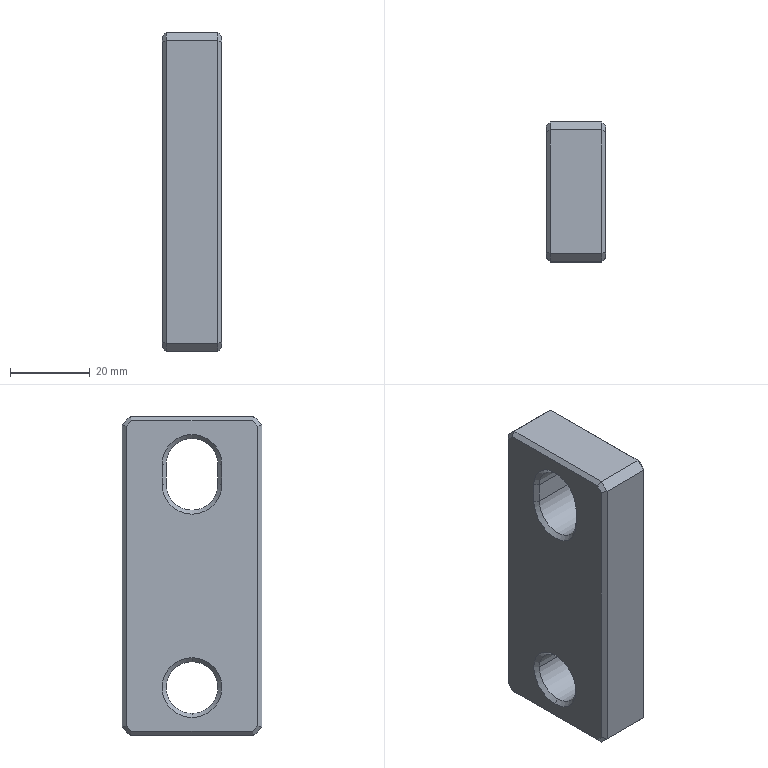Part | Creo | 1 solid | 44 faces | box 15 x 35 x 80 mm | volume 36604 mm3 | plane 32 | cone 8 | cylinder 4 | commonest cylinder face diameters 13 x4
STEP:
#1=CARTESIAN_POINT('',(335.,319.995,12.));
#2=VERTEX_POINT('',#1);
#3=CARTESIAN_POINT('',(336.,320.995,12.));
#4=VERTEX_POINT('',#3);
#5=CARTESIAN_POINT('',(335.,319.995,12.));
#6=DIRECTION('',(0.7071,0.7071,0.));
#7=VECTOR('',#6,1.414);
#8=LINE('',#5,#7);
#9=EDGE_CURVE('',#2,#4,#8,.T.);
#10=ORIENTED_EDGE('',*,*,#9,.F.);
#11=CARTESIAN_POINT('',(335.,327.495,4.5));
#12=VERTEX_POINT('',#11);
#13=CARTESIAN_POINT('',(335.,327.495,12.));
#14=DIRECTION('',(1.,0.,0.));
#15=DIRECTION('',(0.,-1.,0.));
#16=AXIS2_PLACEMENT_3D('',#13,#14,#15);
#17=CIRCLE('',#16,7.5);
#18=EDGE_CURVE('',#2,#12,#17,.T.);
#19=ORIENTED_EDGE('',*,*,#18,.T.);
#20=CARTESIAN_POINT('',(335.,334.995,12.));
#21=VERTEX_POINT('',#20);
#22=CARTESIAN_POINT('',(335.,327.495,12.));
#23=DIRECTION('',(1.,0.,0.));
#24=DIRECTION('',(0.,0.,-1.));
#25=AXIS2_PLACEMENT_3D('',#22,#23,#24);
#26=CIRCLE('',#25,7.5);
#27=EDGE_CURVE('',#12,#21,#26,.T.);
#28=ORIENTED_EDGE('',*,*,#27,.T.);
#29=CARTESIAN_POINT('',(336.,333.995,12.));
#30=VERTEX_POINT('',#29);
#31=CARTESIAN_POINT('',(336.,333.995,12.));
#32=DIRECTION('',(-0.7071,0.7071,0.));
#33=VECTOR('',#32,1.414);
#34=LINE('',#31,#33);
#35=EDGE_CURVE('',#30,#21,#34,.T.);
#36=ORIENTED_EDGE('',*,*,#35,.F.);
#37=CARTESIAN_POINT('',(336.,327.495,5.5));
#38=VERTEX_POINT('',#37);
#39=CARTESIAN_POINT('',(336.,327.495,12.));
#40=DIRECTION('',(1.,0.,0.));
#41=DIRECTION('',(0.,0.,-1.));
#42=AXIS2_PLACEMENT_3D('',#39,#40,#41);
#43=CIRCLE('',#42,6.5);
#44=EDGE_CURVE('',#38,#30,#43,.T.);
#45=ORIENTED_EDGE('',*,*,#44,.F.);
#46=CARTESIAN_POINT('',(336.,327.495,12.));
#47=DIRECTION('',(1.,0.,0.));
#48=DIRECTION('',(0.,-1.,0.));
#49=AXIS2_PLACEMENT_3D('',#46,#47,#48);
#50=CIRCLE('',#49,6.5);
#51=EDGE_CURVE('',#4,#38,#50,.T.);
#52=ORIENTED_EDGE('',*,*,#51,.F.);
#53=EDGE_LOOP('',(#10,#19,#28,#36,#45,#52));
#54=FACE_OUTER_BOUND('',#53,.F.);
#55=CARTESIAN_POINT('',(335.5,327.495,12.));
#56=DIRECTION('',(-1.,0.,0.));
#57=DIRECTION('',(0.,0.,-1.));
#58=AXIS2_PLACEMENT_3D('',#55,#56,#57);
#59=CONICAL_SURFACE('',#58,7.,45.);
#60=ADVANCED_FACE('',(#54),#59,.F.);
#61=CARTESIAN_POINT('',(336.,320.995,17.));
#62=VERTEX_POINT('',#61);
#63=CARTESIAN_POINT('',(335.,319.995,17.));
#64=VERTEX_POINT('',#63);
#65=CARTESIAN_POINT('',(336.,320.995,17.));
#66=DIRECTION('',(-0.7071,-0.7071,0.));
#67=VECTOR('',#66,1.414);
#68=LINE('',#65,#67);
#69=EDGE_CURVE('',#62,#64,#68,.T.);
#70=ORIENTED_EDGE('',*,*,#69,.T.);
#71=CARTESIAN_POINT('',(335.,319.995,12.));
#72=DIRECTION('',(0.,0.,1.));
#73=VECTOR('',#72,5.);
#74=LINE('',#71,#73);
#75=EDGE_CURVE('',#2,#64,#74,.T.);
#76=ORIENTED_EDGE('',*,*,#75,.F.);
#77=ORIENTED_EDGE('',*,*,#9,.T.);
#78=CARTESIAN_POINT('',(336.,320.995,12.));
#79=DIRECTION('',(0.,0.,1.));
#80=VECTOR('',#79,5.);
#81=LINE('',#78,#80);
#82=EDGE_CURVE('',#4,#62,#81,.T.);
#83=ORIENTED_EDGE('',*,*,#82,.T.);
#84=EDGE_LOOP('',(#70,#76,#77,#83));
#85=FACE_OUTER_BOUND('',#84,.F.);
#86=CARTESIAN_POINT('',(335.5,320.495,14.5));
#87=DIRECTION('',(-0.7071,0.7071,0.));
#88=DIRECTION('',(0.7071,0.7071,0.));
#89=AXIS2_PLACEMENT_3D('',#86,#87,#88);
#90=PLANE('',#89);
#91=ADVANCED_FACE('',(#85),#90,.T.);
#92=CARTESIAN_POINT('',(335.,334.995,17.));
#93=VERTEX_POINT('',#92);
#94=CARTESIAN_POINT('',(336.,333.995,17.));
#95=VERTEX_POINT('',#94);
#96=CARTESIAN_POINT('',(335.,334.995,17.));
#97=DIRECTION('',(0.7071,-0.7071,0.));
#98=VECTOR('',#97,1.414);
#99=LINE('',#96,#98);
#100=EDGE_CURVE('',#93,#95,#99,.T.);
#101=ORIENTED_EDGE('',*,*,#100,.F.);
#102=CARTESIAN_POINT('',(335.,327.495,24.5));
#103=VERTEX_POINT('',#102);
#104=CARTESIAN_POINT('',(335.,327.495,17.));
#105=DIRECTION('',(1.,0.,0.));
#106=DIRECTION('',(0.,1.,0.));
#107=AXIS2_PLACEMENT_3D('',#104,#105,#106);
#108=CIRCLE('',#107,7.5);
#109=EDGE_CURVE('',#93,#103,#108,.T.);
#110=ORIENTED_EDGE('',*,*,#109,.T.);
#111=CARTESIAN_POINT('',(335.,327.495,17.));
#112=DIRECTION('',(1.,0.,0.));
#113=DIRECTION('',(0.,0.,1.));
#114=AXIS2_PLACEMENT_3D('',#111,#112,#113);
#115=CIRCLE('',#114,7.5);
#116=EDGE_CURVE('',#103,#64,#115,.T.);
#117=ORIENTED_EDGE('',*,*,#116,.T.);
#118=ORIENTED_EDGE('',*,*,#69,.F.);
#119=CARTESIAN_POINT('',(336.,327.495,23.5));
#120=VERTEX_POINT('',#119);
#121=CARTESIAN_POINT('',(336.,327.495,17.));
#122=DIRECTION('',(1.,0.,0.));
#123=DIRECTION('',(0.,0.,1.));
#124=AXIS2_PLACEMENT_3D('',#121,#122,#123);
#125=CIRCLE('',#124,6.5);
#126=EDGE_CURVE('',#120,#62,#125,.T.);
#127=ORIENTED_EDGE('',*,*,#126,.F.);
#128=CARTESIAN_POINT('',(336.,327.495,17.));
#129=DIRECTION('',(1.,0.,0.));
#130=DIRECTION('',(0.,1.,0.));
#131=AXIS2_PLACEMENT_3D('',#128,#129,#130);
#132=CIRCLE('',#131,6.5);
#133=EDGE_CURVE('',#95,#120,#132,.T.);
#134=ORIENTED_EDGE('',*,*,#133,.F.);
#135=EDGE_LOOP('',(#101,#110,#117,#118,#127,#134));
#136=FACE_OUTER_BOUND('',#135,.F.);
#137=CARTESIAN_POINT('',(335.5,327.495,17.));
#138=DIRECTION('',(-1.,0.,0.));
#139=DIRECTION('',(0.,0.,-1.));
#140=AXIS2_PLACEMENT_3D('',#137,#138,#139);
#141=CONICAL_SURFACE('',#140,7.,45.);
#142=ADVANCED_FACE('',(#136),#141,.F.);
#143=ORIENTED_EDGE('',*,*,#35,.T.);
#144=CARTESIAN_POINT('',(335.,334.995,17.));
#145=DIRECTION('',(0.,0.,-1.));
#146=VECTOR('',#145,5.);
#147=LINE('',#144,#146);
#148=EDGE_CURVE('',#93,#21,#147,.T.);
#149=ORIENTED_EDGE('',*,*,#148,.F.);
#150=ORIENTED_EDGE('',*,*,#100,.T.);
#151=CARTESIAN_POINT('',(336.,333.995,17.));
#152=DIRECTION('',(0.,0.,-1.));
#153=VECTOR('',#152,5.);
#154=LINE('',#151,#153);
#155=EDGE_CURVE('',#95,#30,#154,.T.);
#156=ORIENTED_EDGE('',*,*,#155,.T.);
#157=EDGE_LOOP('',(#143,#149,#150,#156));
#158=FACE_OUTER_BOUND('',#157,.F.);
#159=CARTESIAN_POINT('',(335.5,334.495,14.5));
#160=DIRECTION('',(-0.7071,-0.7071,0.));
#161=DIRECTION('',(0.7071,-0.7071,0.));
#162=AXIS2_PLACEMENT_3D('',#159,#160,#161);
#163=PLANE('',#162);
#164=ADVANCED_FACE('',(#158),#163,.T.);
#165=CARTESIAN_POINT('',(335.,343.995,-48.586));
#166=VERTEX_POINT('',#165);
#167=CARTESIAN_POINT('',(335.,342.581,-50.));
#168=VERTEX_POINT('',#167);
#169=CARTESIAN_POINT('',(335.,343.995,-48.586));
#170=DIRECTION('',(0.,-0.7071,-0.7071));
#171=VECTOR('',#170,2.);
#172=LINE('',#169,#171);
#173=EDGE_CURVE('',#166,#168,#172,.T.);
#174=ORIENTED_EDGE('',*,*,#173,.F.);
#175=CARTESIAN_POINT('',(335.,343.995,26.586));
#176=VERTEX_POINT('',#175);
#177=CARTESIAN_POINT('',(335.,343.995,-48.586));
#178=DIRECTION('',(0.,0.,1.));
#179=VECTOR('',#178,75.172);
#180=LINE('',#177,#179);
#181=EDGE_CURVE('',#166,#176,#180,.T.);
#182=ORIENTED_EDGE('',*,*,#181,.T.);
#183=CARTESIAN_POINT('',(335.,342.581,28.));
#184=VERTEX_POINT('',#183);
#185=CARTESIAN_POINT('',(335.,342.581,28.));
#186=DIRECTION('',(0.,0.7071,-0.7071));
#187=VECTOR('',#186,2.);
#188=LINE('',#185,#187);
#189=EDGE_CURVE('',#184,#176,#188,.T.);
#190=ORIENTED_EDGE('',*,*,#189,.F.);
#191=CARTESIAN_POINT('',(335.,312.41,28.));
#192=VERTEX_POINT('',#191);
#193=CARTESIAN_POINT('',(335.,342.581,28.));
#194=DIRECTION('',(0.,-1.,0.));
#195=VECTOR('',#194,30.172);
#196=LINE('',#193,#195);
#197=EDGE_CURVE('',#184,#192,#196,.T.);
#198=ORIENTED_EDGE('',*,*,#197,.T.);
#199=CARTESIAN_POINT('',(335.,310.995,26.586));
#200=VERTEX_POINT('',#199);
#201=CARTESIAN_POINT('',(335.,310.995,26.586));
#202=DIRECTION('',(0.,0.7071,0.7071));
#203=VECTOR('',#202,2.);
#204=LINE('',#201,#203);
#205=EDGE_CURVE('',#200,#192,#204,.T.);
#206=ORIENTED_EDGE('',*,*,#205,.F.);
#207=CARTESIAN_POINT('',(335.,310.995,-48.586));
#208=VERTEX_POINT('',#207);
#209=CARTESIAN_POINT('',(335.,310.995,26.586));
#210=DIRECTION('',(0.,0.,-1.));
#211=VECTOR('',#210,75.172);
#212=LINE('',#209,#211);
#213=EDGE_CURVE('',#200,#208,#212,.T.);
#214=ORIENTED_EDGE('',*,*,#213,.T.);
#215=CARTESIAN_POINT('',(335.,312.41,-50.));
#216=VERTEX_POINT('',#215);
#217=CARTESIAN_POINT('',(335.,312.41,-50.));
#218=DIRECTION('',(0.,-0.7071,0.7071));
#219=VECTOR('',#218,2.);
#220=LINE('',#217,#219);
#221=EDGE_CURVE('',#216,#208,#220,.T.);
#222=ORIENTED_EDGE('',*,*,#221,.F.);
#223=CARTESIAN_POINT('',(335.,312.41,-50.));
#224=DIRECTION('',(0.,1.,0.));
#225=VECTOR('',#224,30.172);
#226=LINE('',#223,#225);
#227=EDGE_CURVE('',#216,#168,#226,.T.);
#228=ORIENTED_EDGE('',*,*,#227,.T.);
#229=EDGE_LOOP('',(#174,#182,#190,#198,#206,#214,#222,#228));
#230=FACE_OUTER_BOUND('',#229,.F.);
#231=CARTESIAN_POINT('',(335.,334.995,-39.));
#232=VERTEX_POINT('',#231);
#233=CARTESIAN_POINT('',(335.,327.495,-31.5));
#234=VERTEX_POINT('',#233);
#235=CARTESIAN_POINT('',(335.,327.495,-39.));
#236=DIRECTION('',(1.,0.,0.));
#237=DIRECTION('',(0.,1.,0.));
#238=AXIS2_PLACEMENT_3D('',#235,#236,#237);
#239=CIRCLE('',#238,7.5);
#240=EDGE_CURVE('',#232,#234,#239,.T.);
#241=ORIENTED_EDGE('',*,*,#240,.F.);
#242=CARTESIAN_POINT('',(335.,327.495,-46.5));
#243=VERTEX_POINT('',#242);
#244=CARTESIAN_POINT('',(335.,327.495,-39.));
#245=DIRECTION('',(1.,0.,0.));
#246=DIRECTION('',(0.,0.,-1.));
#247=AXIS2_PLACEMENT_3D('',#244,#245,#246);
#248=CIRCLE('',#247,7.5);
#249=EDGE_CURVE('',#243,#232,#248,.T.);
#250=ORIENTED_EDGE('',*,*,#249,.F.);
#251=CARTESIAN_POINT('',(335.,319.995,-39.));
#252=VERTEX_POINT('',#251);
#253=CARTESIAN_POINT('',(335.,327.495,-39.));
#254=DIRECTION('',(1.,0.,0.));
#255=DIRECTION('',(0.,-1.,0.));
#256=AXIS2_PLACEMENT_3D('',#253,#254,#255);
#257=CIRCLE('',#256,7.5);
#258=EDGE_CURVE('',#252,#243,#257,.T.);
#259=ORIENTED_EDGE('',*,*,#258,.F.);
#260=CARTESIAN_POINT('',(335.,327.495,-39.));
#261=DIRECTION('',(1.,0.,0.));
#262=DIRECTION('',(0.,0.,1.));
#263=AXIS2_PLACEMENT_3D('',#260,#261,#262);
#264=CIRCLE('',#263,7.5);
#265=EDGE_CURVE('',#234,#252,#264,.T.);
#266=ORIENTED_EDGE('',*,*,#265,.F.);
#267=EDGE_LOOP('',(#241,#250,#259,#266));
#268=FACE_BOUND('',#267,.F.);
#269=ORIENTED_EDGE('',*,*,#109,.F.);
#270=ORIENTED_EDGE('',*,*,#148,.T.);
#271=ORIENTED_EDGE('',*,*,#27,.F.);
#272=ORIENTED_EDGE('',*,*,#18,.F.);
#273=ORIENTED_EDGE('',*,*,#75,.T.);
#274=ORIENTED_EDGE('',*,*,#116,.F.);
#275=EDGE_LOOP('',(#269,#270,#271,#272,#273,#274));
#276=FACE_BOUND('',#275,.F.);
#277=CARTESIAN_POINT('',(335.,327.495,-11.));
#278=DIRECTION('',(1.,0.,0.));
#279=DIRECTION('',(0.,0.,1.));
#280=AXIS2_PLACEMENT_3D('',#277,#278,#279);
#281=PLANE('',#280);
#282=ADVANCED_FACE('',(#230,#268,#276),#281,.F.);
#283=ORIENTED_EDGE('',*,*,#249,.T.);
#284=ORIENTED_EDGE('',*,*,#240,.T.);
#285=CARTESIAN_POINT('',(336.,327.495,-32.5));
#286=VERTEX_POINT('',#285);
#287=CARTESIAN_POINT('',(336.,327.495,-32.5));
#288=DIRECTION('',(-0.7071,0.,0.7071));
#289=VECTOR('',#288,1.414);
#290=LINE('',#287,#289);
#291=EDGE_CURVE('',#286,#234,#290,.T.);
#292=ORIENTED_EDGE('',*,*,#291,.F.);
#293=CARTESIAN_POINT('',(336.,333.995,-39.));
#294=VERTEX_POINT('',#293);
#295=CARTESIAN_POINT('',(336.,327.495,-39.));
#296=DIRECTION('',(1.,0.,0.));
#297=DIRECTION('',(0.,1.,0.));
#298=AXIS2_PLACEMENT_3D('',#295,#296,#297);
#299=CIRCLE('',#298,6.5);
#300=EDGE_CURVE('',#294,#286,#299,.T.);
#301=ORIENTED_EDGE('',*,*,#300,.F.);
#302=CARTESIAN_POINT('',(336.,327.495,-45.5));
#303=VERTEX_POINT('',#302);
#304=CARTESIAN_POINT('',(336.,327.495,-39.));
#305=DIRECTION('',(1.,0.,0.));
#306=DIRECTION('',(0.,0.,-1.));
#307=AXIS2_PLACEMENT_3D('',#304,#305,#306);
#308=CIRCLE('',#307,6.5);
#309=EDGE_CURVE('',#303,#294,#308,.T.);
#310=ORIENTED_EDGE('',*,*,#309,.F.);
#311=CARTESIAN_POINT('',(336.,327.495,-45.5));
#312=DIRECTION('',(-0.7071,0.,-0.7071));
#313=VECTOR('',#312,1.414);
#314=LINE('',#311,#313);
#315=EDGE_CURVE('',#303,#243,#314,.T.);
#316=ORIENTED_EDGE('',*,*,#315,.T.);
#317=EDGE_LOOP('',(#283,#284,#292,#301,#310,#316));
#318=FACE_OUTER_BOUND('',#317,.F.);
#319=CARTESIAN_POINT('',(335.5,327.495,-39.));
#320=DIRECTION('',(-1.,0.,0.));
#321=DIRECTION('',(0.,0.,-1.));
#322=AXIS2_PLACEMENT_3D('',#319,#320,#321);
#323=CONICAL_SURFACE('',#322,7.,45.);
#324=ADVANCED_FACE('',(#318),#323,.F.);
#325=ORIENTED_EDGE('',*,*,#258,.T.);
#326=ORIENTED_EDGE('',*,*,#315,.F.);
#327=CARTESIAN_POINT('',(336.,320.995,-39.));
#328=VERTEX_POINT('',#327);
#329=CARTESIAN_POINT('',(336.,327.495,-39.));
#330=DIRECTION('',(1.,0.,0.));
#331=DIRECTION('',(0.,-1.,0.));
#332=AXIS2_PLACEMENT_3D('',#329,#330,#331);
#333=CIRCLE('',#332,6.5);
#334=EDGE_CURVE('',#328,#303,#333,.T.);
#335=ORIENTED_EDGE('',*,*,#334,.F.);
#336=CARTESIAN_POINT('',(336.,327.495,-39.));
#337=DIRECTION('',(1.,0.,0.));
#338=DIRECTION('',(0.,0.,1.));
#339=AXIS2_PLACEMENT_3D('',#336,#337,#338);
#340=CIRCLE('',#339,6.5);
#341=EDGE_CURVE('',#286,#328,#340,.T.);
#342=ORIENTED_EDGE('',*,*,#341,.F.);
#343=ORIENTED_EDGE('',*,*,#291,.T.);
#344=ORIENTED_EDGE('',*,*,#265,.T.);
#345=EDGE_LOOP('',(#325,#326,#335,#342,#343,#344));
#346=FACE_OUTER_BOUND('',#345,.F.);
#347=CARTESIAN_POINT('',(335.5,327.495,-39.));
#348=DIRECTION('',(-1.,0.,0.));
#349=DIRECTION('',(0.,0.,-1.));
#350=AXIS2_PLACEMENT_3D('',#347,#348,#349);
#351=CONICAL_SURFACE('',#350,7.,45.);
#352=ADVANCED_FACE('',(#346),#351,.F.);
#353=CARTESIAN_POINT('',(349.,327.495,-45.5));
#354=VERTEX_POINT('',#353);
#355=CARTESIAN_POINT('',(349.,320.995,-39.));
#356=VERTEX_POINT('',#355);
#357=CARTESIAN_POINT('',(349.,327.495,-39.));
#358=DIRECTION('',(-1.,0.,0.));
#359=DIRECTION('',(0.,0.,-1.));
#360=AXIS2_PLACEMENT_3D('',#357,#358,#359);
#361=CIRCLE('',#360,6.5);
#362=EDGE_CURVE('',#354,#356,#361,.T.);
#363=ORIENTED_EDGE('',*,*,#362,.T.);
#364=CARTESIAN_POINT('',(336.,320.995,-39.));
#365=DIRECTION('',(1.,0.,0.));
#366=VECTOR('',#365,13.);
#367=LINE('',#364,#366);
#368=EDGE_CURVE('',#328,#356,#367,.T.);
#369=ORIENTED_EDGE('',*,*,#368,.F.);
#370=ORIENTED_EDGE('',*,*,#334,.T.);
#371=ORIENTED_EDGE('',*,*,#309,.T.);
#372=CARTESIAN_POINT('',(349.,333.995,-39.));
#373=VERTEX_POINT('',#372);
#374=CARTESIAN_POINT('',(336.,333.995,-39.));
#375=DIRECTION('',(1.,0.,0.));
#376=VECTOR('',#375,13.);
#377=LINE('',#374,#376);
#378=EDGE_CURVE('',#294,#373,#377,.T.);
#379=ORIENTED_EDGE('',*,*,#378,.T.);
#380=CARTESIAN_POINT('',(349.,327.495,-39.));
#381=DIRECTION('',(-1.,0.,0.));
#382=DIRECTION('',(0.,1.,0.));
#383=AXIS2_PLACEMENT_3D('',#380,#381,#382);
#384=CIRCLE('',#383,6.5);
#385=EDGE_CURVE('',#373,#354,#384,.T.);
#386=ORIENTED_EDGE('',*,*,#385,.T.);
#387=EDGE_LOOP('',(#363,#369,#370,#371,#379,#386));
#388=FACE_OUTER_BOUND('',#387,.F.);
#389=CARTESIAN_POINT('',(350.,327.495,-39.));
#390=DIRECTION('',(1.,0.,0.));
#391=DIRECTION('',(0.,-1.,0.));
#392=AXIS2_PLACEMENT_3D('',#389,#390,#391);
#393=CYLINDRICAL_SURFACE('',#392,6.5);
#394=ADVANCED_FACE('',(#388),#393,.F.);
#395=CARTESIAN_POINT('',(349.,327.495,-32.5));
#396=VERTEX_POINT('',#395);
#397=CARTESIAN_POINT('',(349.,327.495,-39.));
#398=DIRECTION('',(-1.,0.,0.));
#399=DIRECTION('',(0.,-1.,0.));
#400=AXIS2_PLACEMENT_3D('',#397,#398,#399);
#401=CIRCLE('',#400,6.5);
#402=EDGE_CURVE('',#356,#396,#401,.T.);
#403=ORIENTED_EDGE('',*,*,#402,.F.);
#404=ORIENTED_EDGE('',*,*,#362,.F.);
#405=CARTESIAN_POINT('',(350.,327.495,-46.5));
#406=VERTEX_POINT('',#405);
#407=CARTESIAN_POINT('',(349.,327.495,-45.5));
#408=DIRECTION('',(0.7071,0.,-0.7071));
#409=VECTOR('',#408,1.414);
#410=LINE('',#407,#409);
#411=EDGE_CURVE('',#354,#406,#410,.T.);
#412=ORIENTED_EDGE('',*,*,#411,.T.);
#413=CARTESIAN_POINT('',(350.,319.995,-39.));
#414=VERTEX_POINT('',#413);
#415=CARTESIAN_POINT('',(350.,327.495,-39.));
#416=DIRECTION('',(-1.,0.,0.));
#417=DIRECTION('',(0.,0.,-1.));
#418=AXIS2_PLACEMENT_3D('',#415,#416,#417);
#419=CIRCLE('',#418,7.5);
#420=EDGE_CURVE('',#406,#414,#419,.T.);
#421=ORIENTED_EDGE('',*,*,#420,.T.);
#422=CARTESIAN_POINT('',(350.,327.495,-31.5));
#423=VERTEX_POINT('',#422);
#424=CARTESIAN_POINT('',(350.,327.495,-39.));
#425=DIRECTION('',(-1.,0.,0.));
#426=DIRECTION('',(0.,-1.,0.));
#427=AXIS2_PLACEMENT_3D('',#424,#425,#426);
#428=CIRCLE('',#427,7.5);
#429=EDGE_CURVE('',#414,#423,#428,.T.);
#430=ORIENTED_EDGE('',*,*,#429,.T.);
#431=CARTESIAN_POINT('',(349.,327.495,-32.5));
#432=DIRECTION('',(0.7071,0.,0.7071));
#433=VECTOR('',#432,1.414);
#434=LINE('',#431,#433);
#435=EDGE_CURVE('',#396,#423,#434,.T.);
#436=ORIENTED_EDGE('',*,*,#435,.F.);
#437=EDGE_LOOP('',(#403,#404,#412,#421,#430,#436));
#438=FACE_OUTER_BOUND('',#437,.F.);
#439=CARTESIAN_POINT('',(349.5,327.495,-39.));
#440=DIRECTION('',(1.,0.,0.));
#441=DIRECTION('',(0.,0.,-1.));
#442=AXIS2_PLACEMENT_3D('',#439,#440,#441);
#443=CONICAL_SURFACE('',#442,7.,45.);
#444=ADVANCED_FACE('',(#438),#443,.F.);
#445=CARTESIAN_POINT('',(349.,327.495,-39.));
#446=DIRECTION('',(-1.,0.,0.));
#447=DIRECTION('',(0.,0.,1.));
#448=AXIS2_PLACEMENT_3D('',#445,#446,#447);
#449=CIRCLE('',#448,6.5);
#450=EDGE_CURVE('',#396,#373,#449,.T.);
#451=ORIENTED_EDGE('',*,*,#450,.T.);
#452=ORIENTED_EDGE('',*,*,#378,.F.);
#453=ORIENTED_EDGE('',*,*,#300,.T.);
#454=ORIENTED_EDGE('',*,*,#341,.T.);
#455=ORIENTED_EDGE('',*,*,#368,.T.);
#456=ORIENTED_EDGE('',*,*,#402,.T.);
#457=EDGE_LOOP('',(#451,#452,#453,#454,#455,#456));
#458=FACE_OUTER_BOUND('',#457,.F.);
#459=CARTESIAN_POINT('',(350.,327.495,-39.));
#460=DIRECTION('',(1.,0.,0.));
#461=DIRECTION('',(0.,-1.,0.));
#462=AXIS2_PLACEMENT_3D('',#459,#460,#461);
#463=CYLINDRICAL_SURFACE('',#462,6.5);
#464=ADVANCED_FACE('',(#458),#463,.F.);
#465=ORIENTED_EDGE('',*,*,#450,.F.);
#466=ORIENTED_EDGE('',*,*,#435,.T.);
#467=CARTESIAN_POINT('',(350.,334.995,-39.));
#468=VERTEX_POINT('',#467);
#469=CARTESIAN_POINT('',(350.,327.495,-39.));
#470=DIRECTION('',(-1.,0.,0.));
#471=DIRECTION('',(0.,0.,1.));
#472=AXIS2_PLACEMENT_3D('',#469,#470,#471);
#473=CIRCLE('',#472,7.5);
#474=EDGE_CURVE('',#423,#468,#473,.T.);
#475=ORIENTED_EDGE('',*,*,#474,.T.);
#476=CARTESIAN_POINT('',(350.,327.495,-39.));
#477=DIRECTION('',(-1.,0.,0.));
#478=DIRECTION('',(0.,1.,0.));
#479=AXIS2_PLACEMENT_3D('',#476,#477,#478);
#480=CIRCLE('',#479,7.5);
#481=EDGE_CURVE('',#468,#406,#480,.T.);
#482=ORIENTED_EDGE('',*,*,#481,.T.);
#483=ORIENTED_EDGE('',*,*,#411,.F.);
#484=ORIENTED_EDGE('',*,*,#385,.F.);
#485=EDGE_LOOP('',(#465,#466,#475,#482,#483,#484));
#486=FACE_OUTER_BOUND('',#485,.F.);
#487=CARTESIAN_POINT('',(349.5,327.495,-39.));
#488=DIRECTION('',(1.,0.,0.));
#489=DIRECTION('',(0.,0.,-1.));
#490=AXIS2_PLACEMENT_3D('',#487,#488,#489);
#491=CONICAL_SURFACE('',#490,7.,45.);
#492=ADVANCED_FACE('',(#486),#491,.F.);
#493=CARTESIAN_POINT('',(350.,343.995,26.586));
#494=VERTEX_POINT('',#493);
#495=CARTESIAN_POINT('',(350.,342.581,28.));
#496=VERTEX_POINT('',#495);
#497=CARTESIAN_POINT('',(350.,343.995,26.586));
#498=DIRECTION('',(0.,-0.7071,0.7071));
#499=VECTOR('',#498,2.);
#500=LINE('',#497,#499);
#501=EDGE_CURVE('',#494,#496,#500,.T.);
#502=ORIENTED_EDGE('',*,*,#501,.F.);
#503=CARTESIAN_POINT('',(350.,343.995,-48.586));
#504=VERTEX_POINT('',#503);
#505=CARTESIAN_POINT('',(350.,343.995,26.586));
#506=DIRECTION('',(0.,0.,-1.));
#507=VECTOR('',#506,75.172);
#508=LINE('',#505,#507);
#509=EDGE_CURVE('',#494,#504,#508,.T.);
#510=ORIENTED_EDGE('',*,*,#509,.T.);
#511=CARTESIAN_POINT('',(350.,342.581,-50.));
#512=VERTEX_POINT('',#511);
#513=CARTESIAN_POINT('',(350.,342.581,-50.));
#514=DIRECTION('',(0.,0.7071,0.7071));
#515=VECTOR('',#514,2.);
#516=LINE('',#513,#515);
#517=EDGE_CURVE('',#512,#504,#516,.T.);
#518=ORIENTED_EDGE('',*,*,#517,.F.);
#519=CARTESIAN_POINT('',(350.,312.41,-50.));
#520=VERTEX_POINT('',#519);
#521=CARTESIAN_POINT('',(350.,342.581,-50.));
#522=DIRECTION('',(0.,-1.,0.));
#523=VECTOR('',#522,30.172);
#524=LINE('',#521,#523);
#525=EDGE_CURVE('',#512,#520,#524,.T.);
#526=ORIENTED_EDGE('',*,*,#525,.T.);
#527=CARTESIAN_POINT('',(350.,310.995,-48.586));
#528=VERTEX_POINT('',#527);
#529=CARTESIAN_POINT('',(350.,310.995,-48.586));
#530=DIRECTION('',(0.,0.7071,-0.7071));
#531=VECTOR('',#530,2.);
#532=LINE('',#529,#531);
#533=EDGE_CURVE('',#528,#520,#532,.T.);
#534=ORIENTED_EDGE('',*,*,#533,.F.);
#535=CARTESIAN_POINT('',(350.,310.995,26.586));
#536=VERTEX_POINT('',#535);
#537=CARTESIAN_POINT('',(350.,310.995,-48.586));
#538=DIRECTION('',(0.,0.,1.));
#539=VECTOR('',#538,75.172);
#540=LINE('',#537,#539);
#541=EDGE_CURVE('',#528,#536,#540,.T.);
#542=ORIENTED_EDGE('',*,*,#541,.T.);
#543=CARTESIAN_POINT('',(350.,312.41,28.));
#544=VERTEX_POINT('',#543);
#545=CARTESIAN_POINT('',(350.,312.41,28.));
#546=DIRECTION('',(0.,-0.7071,-0.7071));
#547=VECTOR('',#546,2.);
#548=LINE('',#545,#547);
#549=EDGE_CURVE('',#544,#536,#548,.T.);
#550=ORIENTED_EDGE('',*,*,#549,.F.);
#551=CARTESIAN_POINT('',(350.,312.41,28.));
#552=DIRECTION('',(0.,1.,0.));
#553=VECTOR('',#552,30.172);
#554=LINE('',#551,#553);
#555=EDGE_CURVE('',#544,#496,#554,.T.);
#556=ORIENTED_EDGE('',*,*,#555,.T.);
#557=EDGE_LOOP('',(#502,#510,#518,#526,#534,#542,#550,#556));
#558=FACE_OUTER_BOUND('',#557,.F.);
#559=ORIENTED_EDGE('',*,*,#429,.F.);
#560=ORIENTED_EDGE('',*,*,#420,.F.);
#561=ORIENTED_EDGE('',*,*,#481,.F.);
#562=ORIENTED_EDGE('',*,*,#474,.F.);
#563=EDGE_LOOP('',(#559,#560,#561,#562));
#564=FACE_BOUND('',#563,.F.);
#565=CARTESIAN_POINT('',(350.,319.995,17.));
#566=VERTEX_POINT('',#565);
#567=CARTESIAN_POINT('',(350.,327.495,24.5));
#568=VERTEX_POINT('',#567);
#569=CARTESIAN_POINT('',(350.,327.495,17.));
#570=DIRECTION('',(-1.,0.,0.));
#571=DIRECTION('',(0.,-1.,0.));
#572=AXIS2_PLACEMENT_3D('',#569,#570,#571);
#573=CIRCLE('',#572,7.5);
#574=EDGE_CURVE('',#566,#568,#573,.T.);
#575=ORIENTED_EDGE('',*,*,#574,.F.);
#576=CARTESIAN_POINT('',(350.,319.995,12.));
#577=VERTEX_POINT('',#576);
#578=CARTESIAN_POINT('',(350.,319.995,17.));
#579=DIRECTION('',(0.,0.,-1.));
#580=VECTOR('',#579,5.);
#581=LINE('',#578,#580);
#582=EDGE_CURVE('',#566,#577,#581,.T.);
#583=ORIENTED_EDGE('',*,*,#582,.T.);
#584=CARTESIAN_POINT('',(350.,327.495,4.5));
#585=VERTEX_POINT('',#584);
#586=CARTESIAN_POINT('',(350.,327.495,12.));
#587=DIRECTION('',(-1.,0.,0.));
#588=DIRECTION('',(0.,0.,-1.));
#589=AXIS2_PLACEMENT_3D('',#586,#587,#588);
#590=CIRCLE('',#589,7.5);
#591=EDGE_CURVE('',#585,#577,#590,.T.);
#592=ORIENTED_EDGE('',*,*,#591,.F.);
#593=CARTESIAN_POINT('',(350.,334.995,12.));
#594=VERTEX_POINT('',#593);
#595=CARTESIAN_POINT('',(350.,327.495,12.));
#596=DIRECTION('',(-1.,0.,0.));
#597=DIRECTION('',(0.,1.,0.));
#598=AXIS2_PLACEMENT_3D('',#595,#596,#597);
#599=CIRCLE('',#598,7.5);
#600=EDGE_CURVE('',#594,#585,#599,.T.);
#601=ORIENTED_EDGE('',*,*,#600,.F.);
#602=CARTESIAN_POINT('',(350.,334.995,17.));
#603=VERTEX_POINT('',#602);
#604=CARTESIAN_POINT('',(350.,334.995,12.));
#605=DIRECTION('',(0.,0.,1.));
#606=VECTOR('',#605,5.);
#607=LINE('',#604,#606);
#608=EDGE_CURVE('',#594,#603,#607,.T.);
#609=ORIENTED_EDGE('',*,*,#608,.T.);
#610=CARTESIAN_POINT('',(350.,327.495,17.));
#611=DIRECTION('',(-1.,0.,0.));
#612=DIRECTION('',(0.,0.,1.));
#613=AXIS2_PLACEMENT_3D('',#610,#611,#612);
#614=CIRCLE('',#613,7.5);
#615=EDGE_CURVE('',#568,#603,#614,.T.);
#616=ORIENTED_EDGE('',*,*,#615,.F.);
#617=EDGE_LOOP('',(#575,#583,#592,#601,#609,#616));
#618=FACE_BOUND('',#617,.F.);
#619=CARTESIAN_POINT('',(350.,327.495,-11.));
#620=DIRECTION('',(1.,0.,0.));
#621=DIRECTION('',(0.,0.,1.));
#622=AXIS2_PLACEMENT_3D('',#619,#620,#621);
#623=PLANE('',#622);
#624=ADVANCED_FACE('',(#558,#564,#618),#623,.T.);
#625=CARTESIAN_POINT('',(349.,320.995,17.));
#626=VERTEX_POINT('',#625);
#627=CARTESIAN_POINT('',(350.,319.995,17.));
#628=DIRECTION('',(-0.7071,0.7071,0.));
#629=VECTOR('',#628,1.414);
#630=LINE('',#627,#629);
#631=EDGE_CURVE('',#566,#626,#630,.T.);
#632=ORIENTED_EDGE('',*,*,#631,.F.);
#633=ORIENTED_EDGE('',*,*,#574,.T.);
#634=ORIENTED_EDGE('',*,*,#615,.T.);
#635=CARTESIAN_POINT('',(349.,333.995,17.));
#636=VERTEX_POINT('',#635);
#637=CARTESIAN_POINT('',(349.,333.995,17.));
#638=DIRECTION('',(0.7071,0.7071,0.));
#639=VECTOR('',#638,1.414);
#640=LINE('',#637,#639);
#641=EDGE_CURVE('',#636,#603,#640,.T.);
#642=ORIENTED_EDGE('',*,*,#641,.F.);
#643=CARTESIAN_POINT('',(349.,327.495,23.5));
#644=VERTEX_POINT('',#643);
#645=CARTESIAN_POINT('',(349.,327.495,17.));
#646=DIRECTION('',(-1.,0.,0.));
#647=DIRECTION('',(0.,0.,1.));
#648=AXIS2_PLACEMENT_3D('',#645,#646,#647);
#649=CIRCLE('',#648,6.5);
#650=EDGE_CURVE('',#644,#636,#649,.T.);
#651=ORIENTED_EDGE('',*,*,#650,.F.);
#652=CARTESIAN_POINT('',(349.,327.495,17.));
#653=DIRECTION('',(-1.,0.,0.));
#654=DIRECTION('',(0.,-1.,0.));
#655=AXIS2_PLACEMENT_3D('',#652,#653,#654);
#656=CIRCLE('',#655,6.5);
#657=EDGE_CURVE('',#626,#644,#656,.T.);
#658=ORIENTED_EDGE('',*,*,#657,.F.);
#659=EDGE_LOOP('',(#632,#633,#634,#642,#651,#658));
#660=FACE_OUTER_BOUND('',#659,.F.);
#661=CARTESIAN_POINT('',(349.5,327.495,17.));
#662=DIRECTION('',(1.,0.,0.));
#663=DIRECTION('',(0.,0.,-1.));
#664=AXIS2_PLACEMENT_3D('',#661,#662,#663);
#665=CONICAL_SURFACE('',#664,7.,45.);
#666=ADVANCED_FACE('',(#660),#665,.F.);
#667=CARTESIAN_POINT('',(349.,320.995,12.));
#668=VERTEX_POINT('',#667);
#669=CARTESIAN_POINT('',(349.,320.995,12.));
#670=DIRECTION('',(0.7071,-0.7071,0.));
#671=VECTOR('',#670,1.414);
#672=LINE('',#669,#671);
#673=EDGE_CURVE('',#668,#577,#672,.T.);
#674=ORIENTED_EDGE('',*,*,#673,.T.);
#675=ORIENTED_EDGE('',*,*,#582,.F.);
#676=ORIENTED_EDGE('',*,*,#631,.T.);
#677=CARTESIAN_POINT('',(349.,320.995,17.));
#678=DIRECTION('',(0.,0.,-1.));
#679=VECTOR('',#678,5.);
#680=LINE('',#677,#679);
#681=EDGE_CURVE('',#626,#668,#680,.T.);
#682=ORIENTED_EDGE('',*,*,#681,.T.);
#683=EDGE_LOOP('',(#674,#675,#676,#682));
#684=FACE_OUTER_BOUND('',#683,.F.);
#685=CARTESIAN_POINT('',(349.5,320.495,14.5));
#686=DIRECTION('',(0.7071,0.7071,0.));
#687=DIRECTION('',(-0.7071,0.7071,0.));
#688=AXIS2_PLACEMENT_3D('',#685,#686,#687);
#689=PLANE('',#688);
#690=ADVANCED_FACE('',(#684),#689,.T.);
#691=CARTESIAN_POINT('',(349.,333.995,12.));
#692=VERTEX_POINT('',#691);
#693=CARTESIAN_POINT('',(350.,334.995,12.));
#694=DIRECTION('',(-0.7071,-0.7071,0.));
#695=VECTOR('',#694,1.414);
#696=LINE('',#693,#695);
#697=EDGE_CURVE('',#594,#692,#696,.T.);
#698=ORIENTED_EDGE('',*,*,#697,.F.);
#699=ORIENTED_EDGE('',*,*,#600,.T.);
#700=ORIENTED_EDGE('',*,*,#591,.T.);
#701=ORIENTED_EDGE('',*,*,#673,.F.);
#702=CARTESIAN_POINT('',(349.,327.495,5.5));
#703=VERTEX_POINT('',#702);
#704=CARTESIAN_POINT('',(349.,327.495,12.));
#705=DIRECTION('',(-1.,0.,0.));
#706=DIRECTION('',(0.,0.,-1.));
#707=AXIS2_PLACEMENT_3D('',#704,#705,#706);
#708=CIRCLE('',#707,6.5);
#709=EDGE_CURVE('',#703,#668,#708,.T.);
#710=ORIENTED_EDGE('',*,*,#709,.F.);
#711=CARTESIAN_POINT('',(349.,327.495,12.));
#712=DIRECTION('',(-1.,0.,0.));
#713=DIRECTION('',(0.,1.,0.));
#714=AXIS2_PLACEMENT_3D('',#711,#712,#713);
#715=CIRCLE('',#714,6.5);
#716=EDGE_CURVE('',#692,#703,#715,.T.);
#717=ORIENTED_EDGE('',*,*,#716,.F.);
#718=EDGE_LOOP('',(#698,#699,#700,#701,#710,#717));
#719=FACE_OUTER_BOUND('',#718,.F.);
#720=CARTESIAN_POINT('',(349.5,327.495,12.));
#721=DIRECTION('',(1.,0.,0.));
#722=DIRECTION('',(0.,0.,-1.));
#723=AXIS2_PLACEMENT_3D('',#720,#721,#722);
#724=CONICAL_SURFACE('',#723,7.,45.);
#725=ADVANCED_FACE('',(#719),#724,.F.);
#726=ORIENTED_EDGE('',*,*,#641,.T.);
#727=ORIENTED_EDGE('',*,*,#608,.F.);
#728=ORIENTED_EDGE('',*,*,#697,.T.);
#729=CARTESIAN_POINT('',(349.,333.995,12.));
#730=DIRECTION('',(0.,0.,1.));
#731=VECTOR('',#730,5.);
#732=LINE('',#729,#731);
#733=EDGE_CURVE('',#692,#636,#732,.T.);
#734=ORIENTED_EDGE('',*,*,#733,.T.);
#735=EDGE_LOOP('',(#726,#727,#728,#734));
#736=FACE_OUTER_BOUND('',#735,.F.);
#737=CARTESIAN_POINT('',(349.5,334.495,14.5));
#738=DIRECTION('',(0.7071,-0.7071,0.));
#739=DIRECTION('',(-0.7071,-0.7071,0.));
#740=AXIS2_PLACEMENT_3D('',#737,#738,#739);
#741=PLANE('',#740);
#742=ADVANCED_FACE('',(#736),#741,.T.);
#743=CARTESIAN_POINT('',(336.,333.995,17.));
#744=DIRECTION('',(1.,0.,0.));
#745=VECTOR('',#744,13.);
#746=LINE('',#743,#745);
#747=EDGE_CURVE('',#95,#636,#746,.T.);
#748=ORIENTED_EDGE('',*,*,#747,.T.);
#749=ORIENTED_EDGE('',*,*,#733,.F.);
#750=CARTESIAN_POINT('',(349.,333.995,12.));
#751=DIRECTION('',(-1.,0.,0.));
#752=VECTOR('',#751,13.);
#753=LINE('',#750,#752);
#754=EDGE_CURVE('',#692,#30,#753,.T.);
#755=ORIENTED_EDGE('',*,*,#754,.T.);
#756=ORIENTED_EDGE('',*,*,#155,.F.);
#757=EDGE_LOOP('',(#748,#749,#755,#756));
#758=FACE_OUTER_BOUND('',#757,.F.);
#759=CARTESIAN_POINT('',(350.,333.995,12.));
#760=DIRECTION('',(0.,1.,0.));
#761=DIRECTION('',(0.,0.,1.));
#762=AXIS2_PLACEMENT_3D('',#759,#760,#761);
#763=PLANE('',#762);
#764=ADVANCED_FACE('',(#758),#763,.F.);
#765=CARTESIAN_POINT('',(349.,320.995,17.));
#766=DIRECTION('',(-1.,0.,0.));
#767=VECTOR('',#766,13.);
#768=LINE('',#765,#767);
#769=EDGE_CURVE('',#626,#62,#768,.T.);
#770=ORIENTED_EDGE('',*,*,#769,.F.);
#771=ORIENTED_EDGE('',*,*,#657,.T.);
#772=ORIENTED_EDGE('',*,*,#650,.T.);
#773=ORIENTED_EDGE('',*,*,#747,.F.);
#774=ORIENTED_EDGE('',*,*,#133,.T.);
#775=ORIENTED_EDGE('',*,*,#126,.T.);
#776=EDGE_LOOP('',(#770,#771,#772,#773,#774,#775));
#777=FACE_OUTER_BOUND('',#776,.F.);
#778=CARTESIAN_POINT('',(350.,327.495,17.));
#779=DIRECTION('',(1.,0.,0.));
#780=DIRECTION('',(0.,-1.,0.));
#781=AXIS2_PLACEMENT_3D('',#778,#779,#780);
#782=CYLINDRICAL_SURFACE('',#781,6.5);
#783=ADVANCED_FACE('',(#777),#782,.F.);
#784=CARTESIAN_POINT('',(336.,320.995,12.));
#785=DIRECTION('',(1.,0.,0.));
#786=VECTOR('',#785,13.);
#787=LINE('',#784,#786);
#788=EDGE_CURVE('',#4,#668,#787,.T.);
#789=ORIENTED_EDGE('',*,*,#788,.T.);
#790=ORIENTED_EDGE('',*,*,#681,.F.);
#791=ORIENTED_EDGE('',*,*,#769,.T.);
#792=ORIENTED_EDGE('',*,*,#82,.F.);
#793=EDGE_LOOP('',(#789,#790,#791,#792));
#794=FACE_OUTER_BOUND('',#793,.F.);
#795=CARTESIAN_POINT('',(350.,320.995,17.));
#796=DIRECTION('',(0.,-1.,0.));
#797=DIRECTION('',(0.,0.,-1.));
#798=AXIS2_PLACEMENT_3D('',#795,#796,#797);
#799=PLANE('',#798);
#800=ADVANCED_FACE('',(#794),#799,.F.);
#801=ORIENTED_EDGE('',*,*,#754,.F.);
#802=ORIENTED_EDGE('',*,*,#716,.T.);
#803=ORIENTED_EDGE('',*,*,#709,.T.);
#804=ORIENTED_EDGE('',*,*,#788,.F.);
#805=ORIENTED_EDGE('',*,*,#51,.T.);
#806=ORIENTED_EDGE('',*,*,#44,.T.);
#807=EDGE_LOOP('',(#801,#802,#803,#804,#805,#806));
#808=FACE_OUTER_BOUND('',#807,.F.);
#809=CARTESIAN_POINT('',(350.,327.495,12.));
#810=DIRECTION('',(1.,0.,0.));
#811=DIRECTION('',(0.,-1.,0.));
#812=AXIS2_PLACEMENT_3D('',#809,#810,#811);
#813=CYLINDRICAL_SURFACE('',#812,6.5);
#814=ADVANCED_FACE('',(#808),#813,.F.);
#815=CARTESIAN_POINT('',(349.,344.995,27.));
#816=VERTEX_POINT('',#815);
#817=CARTESIAN_POINT('',(350.,343.995,26.586));
#818=DIRECTION('',(-0.6786,0.6786,0.2811));
#819=VECTOR('',#818,1.474);
#820=LINE('',#817,#819);
#821=EDGE_CURVE('',#494,#816,#820,.T.);
#822=ORIENTED_EDGE('',*,*,#821,.F.);
#823=ORIENTED_EDGE('',*,*,#501,.T.);
#824=CARTESIAN_POINT('',(349.,342.995,29.));
#825=VERTEX_POINT('',#824);
#826=CARTESIAN_POINT('',(350.,342.581,28.));
#827=DIRECTION('',(-0.6786,0.2811,0.6786));
#828=VECTOR('',#827,1.474);
#829=LINE('',#826,#828);
#830=EDGE_CURVE('',#496,#825,#829,.T.);
#831=ORIENTED_EDGE('',*,*,#830,.T.);
#832=CARTESIAN_POINT('',(349.,342.995,29.));
#833=DIRECTION('',(0.,0.7071,-0.7071));
#834=VECTOR('',#833,2.828);
#835=LINE('',#832,#834);
#836=EDGE_CURVE('',#825,#816,#835,.T.);
#837=ORIENTED_EDGE('',*,*,#836,.T.);
#838=EDGE_LOOP('',(#822,#823,#831,#837));
#839=FACE_OUTER_BOUND('',#838,.F.);
#840=CARTESIAN_POINT('',(349.5,343.642,27.646));
#841=DIRECTION('',(0.7071,0.5,0.5));
#842=DIRECTION('',(-0.7071,0.5,0.5));
#843=AXIS2_PLACEMENT_3D('',#840,#841,#842);
#844=PLANE('',#843);
#845=ADVANCED_FACE('',(#839),#844,.T.);
#846=ORIENTED_EDGE('',*,*,#821,.T.);
#847=CARTESIAN_POINT('',(349.,344.995,-49.));
#848=VERTEX_POINT('',#847);
#849=CARTESIAN_POINT('',(349.,344.995,27.));
#850=DIRECTION('',(0.,0.,-1.));
#851=VECTOR('',#850,76.);
#852=LINE('',#849,#851);
#853=EDGE_CURVE('',#816,#848,#852,.T.);
#854=ORIENTED_EDGE('',*,*,#853,.T.);
#855=CARTESIAN_POINT('',(350.,343.995,-48.586));
#856=DIRECTION('',(-0.6786,0.6786,-0.2811));
#857=VECTOR('',#856,1.474);
#858=LINE('',#855,#857);
#859=EDGE_CURVE('',#504,#848,#858,.T.);
#860=ORIENTED_EDGE('',*,*,#859,.F.);
#861=ORIENTED_EDGE('',*,*,#509,.F.);
#862=EDGE_LOOP('',(#846,#854,#860,#861));
#863=FACE_OUTER_BOUND('',#862,.F.);
#864=CARTESIAN_POINT('',(349.5,344.495,-11.));
#865=DIRECTION('',(0.7071,0.7071,0.));
#866=DIRECTION('',(-0.7071,0.7071,0.));
#867=AXIS2_PLACEMENT_3D('',#864,#865,#866);
#868=PLANE('',#867);
#869=ADVANCED_FACE('',(#863),#868,.T.);
#870=CARTESIAN_POINT('',(336.,344.995,27.));
#871=VERTEX_POINT('',#870);
#872=CARTESIAN_POINT('',(336.,344.995,27.));
#873=DIRECTION('',(1.,0.,0.));
#874=VECTOR('',#873,13.);
#875=LINE('',#872,#874);
#876=EDGE_CURVE('',#871,#816,#875,.T.);
#877=ORIENTED_EDGE('',*,*,#876,.F.);
#878=CARTESIAN_POINT('',(336.,344.995,-49.));
#879=VERTEX_POINT('',#878);
#880=CARTESIAN_POINT('',(336.,344.995,-49.));
#881=DIRECTION('',(0.,0.,1.));
#882=VECTOR('',#881,76.);
#883=LINE('',#880,#882);
#884=EDGE_CURVE('',#879,#871,#883,.T.);
#885=ORIENTED_EDGE('',*,*,#884,.F.);
#886=CARTESIAN_POINT('',(336.,344.995,-49.));
#887=DIRECTION('',(1.,0.,0.));
#888=VECTOR('',#887,13.);
#889=LINE('',#886,#888);
#890=EDGE_CURVE('',#879,#848,#889,.T.);
#891=ORIENTED_EDGE('',*,*,#890,.T.);
#892=ORIENTED_EDGE('',*,*,#853,.F.);
#893=EDGE_LOOP('',(#877,#885,#891,#892));
#894=FACE_OUTER_BOUND('',#893,.F.);
#895=CARTESIAN_POINT('',(335.,344.995,-51.));
#896=DIRECTION('',(0.,1.,0.));
#897=DIRECTION('',(0.,0.,1.));
#898=AXIS2_PLACEMENT_3D('',#895,#896,#897);
#899=PLANE('',#898);
#900=ADVANCED_FACE('',(#894),#899,.T.);
#901=CARTESIAN_POINT('',(336.,342.995,29.));
#902=VERTEX_POINT('',#901);
#903=CARTESIAN_POINT('',(336.,342.995,29.));
#904=DIRECTION('',(1.,0.,0.));
#905=VECTOR('',#904,13.);
#906=LINE('',#903,#905);
#907=EDGE_CURVE('',#902,#825,#906,.T.);
#908=ORIENTED_EDGE('',*,*,#907,.F.);
#909=CARTESIAN_POINT('',(336.,344.995,27.));
#910=DIRECTION('',(0.,-0.7071,0.7071));
#911=VECTOR('',#910,2.828);
#912=LINE('',#909,#911);
#913=EDGE_CURVE('',#871,#902,#912,.T.);
#914=ORIENTED_EDGE('',*,*,#913,.F.);
#915=ORIENTED_EDGE('',*,*,#876,.T.);
#916=ORIENTED_EDGE('',*,*,#836,.F.);
#917=EDGE_LOOP('',(#908,#914,#915,#916));
#918=FACE_OUTER_BOUND('',#917,.F.);
#919=CARTESIAN_POINT('',(342.5,343.995,28.));
#920=DIRECTION('',(0.,0.7071,0.7071));
#921=DIRECTION('',(0.,0.7071,-0.7071));
#922=AXIS2_PLACEMENT_3D('',#919,#920,#921);
#923=PLANE('',#922);
#924=ADVANCED_FACE('',(#918),#923,.T.);
#925=CARTESIAN_POINT('',(336.,311.995,29.));
#926=VERTEX_POINT('',#925);
#927=CARTESIAN_POINT('',(349.,311.995,29.));
#928=VERTEX_POINT('',#927);
#929=CARTESIAN_POINT('',(336.,311.995,29.));
#930=DIRECTION('',(1.,0.,0.));
#931=VECTOR('',#930,13.);
#932=LINE('',#929,#931);
#933=EDGE_CURVE('',#926,#928,#932,.T.);
#934=ORIENTED_EDGE('',*,*,#933,.F.);
#935=CARTESIAN_POINT('',(336.,342.995,29.));
#936=DIRECTION('',(0.,-1.,0.));
#937=VECTOR('',#936,31.);
#938=LINE('',#935,#937);
#939=EDGE_CURVE('',#902,#926,#938,.T.);
#940=ORIENTED_EDGE('',*,*,#939,.F.);
#941=ORIENTED_EDGE('',*,*,#907,.T.);
#942=CARTESIAN_POINT('',(349.,311.995,29.));
#943=DIRECTION('',(0.,1.,0.));
#944=VECTOR('',#943,31.);
#945=LINE('',#942,#944);
#946=EDGE_CURVE('',#928,#825,#945,.T.);
#947=ORIENTED_EDGE('',*,*,#946,.F.);
#948=EDGE_LOOP('',(#934,#940,#941,#947));
#949=FACE_OUTER_BOUND('',#948,.F.);
#950=CARTESIAN_POINT('',(335.,344.995,29.));
#951=DIRECTION('',(0.,0.,1.));
#952=DIRECTION('',(0.,-1.,0.));
#953=AXIS2_PLACEMENT_3D('',#950,#951,#952);
#954=PLANE('',#953);
#955=ADVANCED_FACE('',(#949),#954,.T.);
#956=CARTESIAN_POINT('',(336.,309.995,27.));
#957=VERTEX_POINT('',#956);
#958=CARTESIAN_POINT('',(349.,309.995,27.));
#959=VERTEX_POINT('',#958);
#960=CARTESIAN_POINT('',(336.,309.995,27.));
#961=DIRECTION('',(1.,0.,0.));
#962=VECTOR('',#961,13.);
#963=LINE('',#960,#962);
#964=EDGE_CURVE('',#957,#959,#963,.T.);
#965=ORIENTED_EDGE('',*,*,#964,.F.);
#966=CARTESIAN_POINT('',(336.,311.995,29.));
#967=DIRECTION('',(0.,-0.7071,-0.7071));
#968=VECTOR('',#967,2.828);
#969=LINE('',#966,#968);
#970=EDGE_CURVE('',#926,#957,#969,.T.);
#971=ORIENTED_EDGE('',*,*,#970,.F.);
#972=ORIENTED_EDGE('',*,*,#933,.T.);
#973=CARTESIAN_POINT('',(349.,309.995,27.));
#974=DIRECTION('',(0.,0.7071,0.7071));
#975=VECTOR('',#974,2.828);
#976=LINE('',#973,#975);
#977=EDGE_CURVE('',#959,#928,#976,.T.);
#978=ORIENTED_EDGE('',*,*,#977,.F.);
#979=EDGE_LOOP('',(#965,#971,#972,#978));
#980=FACE_OUTER_BOUND('',#979,.F.);
#981=CARTESIAN_POINT('',(342.5,310.995,28.));
#982=DIRECTION('',(0.,-0.7071,0.7071));
#983=DIRECTION('',(0.,0.7071,0.7071));
#984=AXIS2_PLACEMENT_3D('',#981,#982,#983);
#985=PLANE('',#984);
#986=ADVANCED_FACE('',(#980),#985,.T.);
#987=CARTESIAN_POINT('',(336.,309.995,-49.));
#988=VERTEX_POINT('',#987);
#989=CARTESIAN_POINT('',(349.,309.995,-49.));
#990=VERTEX_POINT('',#989);
#991=CARTESIAN_POINT('',(336.,309.995,-49.));
#992=DIRECTION('',(1.,0.,0.));
#993=VECTOR('',#992,13.);
#994=LINE('',#991,#993);
#995=EDGE_CURVE('',#988,#990,#994,.T.);
#996=ORIENTED_EDGE('',*,*,#995,.F.);
#997=CARTESIAN_POINT('',(336.,309.995,27.));
#998=DIRECTION('',(0.,0.,-1.));
#999=VECTOR('',#998,76.);
#1000=LINE('',#997,#999);
#1001=EDGE_CURVE('',#957,#988,#1000,.T.);
#1002=ORIENTED_EDGE('',*,*,#1001,.F.);
#1003=ORIENTED_EDGE('',*,*,#964,.T.);
#1004=CARTESIAN_POINT('',(349.,309.995,-49.));
#1005=DIRECTION('',(0.,0.,1.));
#1006=VECTOR('',#1005,76.);
#1007=LINE('',#1004,#1006);
#1008=EDGE_CURVE('',#990,#959,#1007,.T.);
#1009=ORIENTED_EDGE('',*,*,#1008,.F.);
#1010=EDGE_LOOP('',(#996,#1002,#1003,#1009));
#1011=FACE_OUTER_BOUND('',#1010,.F.);
#1012=CARTESIAN_POINT('',(335.,309.995,29.));
#1013=DIRECTION('',(0.,-1.,0.));
#1014=DIRECTION('',(0.,0.,-1.));
#1015=AXIS2_PLACEMENT_3D('',#1012,#1013,#1014);
#1016=PLANE('',#1015);
#1017=ADVANCED_FACE('',(#1011),#1016,.T.);
#1018=CARTESIAN_POINT('',(336.,311.995,-51.));
#1019=VERTEX_POINT('',#1018);
#1020=CARTESIAN_POINT('',(349.,311.995,-51.));
#1021=VERTEX_POINT('',#1020);
#1022=CARTESIAN_POINT('',(336.,311.995,-51.));
#1023=DIRECTION('',(1.,0.,0.));
#1024=VECTOR('',#1023,13.);
#1025=LINE('',#1022,#1024);
#1026=EDGE_CURVE('',#1019,#1021,#1025,.T.);
#1027=ORIENTED_EDGE('',*,*,#1026,.F.);
#1028=CARTESIAN_POINT('',(336.,309.995,-49.));
#1029=DIRECTION('',(0.,0.7071,-0.7071));
#1030=VECTOR('',#1029,2.828);
#1031=LINE('',#1028,#1030);
#1032=EDGE_CURVE('',#988,#1019,#1031,.T.);
#1033=ORIENTED_EDGE('',*,*,#1032,.F.);
#1034=ORIENTED_EDGE('',*,*,#995,.T.);
#1035=CARTESIAN_POINT('',(349.,311.995,-51.));
#1036=DIRECTION('',(0.,-0.7071,0.7071));
#1037=VECTOR('',#1036,2.828);
#1038=LINE('',#1035,#1037);
#1039=EDGE_CURVE('',#1021,#990,#1038,.T.);
#1040=ORIENTED_EDGE('',*,*,#1039,.F.);
#1041=EDGE_LOOP('',(#1027,#1033,#1034,#1040));
#1042=FACE_OUTER_BOUND('',#1041,.F.);
#1043=CARTESIAN_POINT('',(342.5,310.995,-50.));
#1044=DIRECTION('',(0.,-0.7071,-0.7071));
#1045=DIRECTION('',(0.,-0.7071,0.7071));
#1046=AXIS2_PLACEMENT_3D('',#1043,#1044,#1045);
#1047=PLANE('',#1046);
#1048=ADVANCED_FACE('',(#1042),#1047,.T.);
#1049=CARTESIAN_POINT('',(336.,342.995,-51.));
#1050=VERTEX_POINT('',#1049);
#1051=CARTESIAN_POINT('',(349.,342.995,-51.));
#1052=VERTEX_POINT('',#1051);
#1053=CARTESIAN_POINT('',(336.,342.995,-51.));
#1054=DIRECTION('',(1.,0.,0.));
#1055=VECTOR('',#1054,13.);
#1056=LINE('',#1053,#1055);
#1057=EDGE_CURVE('',#1050,#1052,#1056,.T.);
#1058=ORIENTED_EDGE('',*,*,#1057,.F.);
#1059=CARTESIAN_POINT('',(336.,311.995,-51.));
#1060=DIRECTION('',(0.,1.,0.));
#1061=VECTOR('',#1060,31.);
#1062=LINE('',#1059,#1061);
#1063=EDGE_CURVE('',#1019,#1050,#1062,.T.);
#1064=ORIENTED_EDGE('',*,*,#1063,.F.);
#1065=ORIENTED_EDGE('',*,*,#1026,.T.);
#1066=CARTESIAN_POINT('',(349.,342.995,-51.));
#1067=DIRECTION('',(0.,-1.,0.));
#1068=VECTOR('',#1067,31.);
#1069=LINE('',#1066,#1068);
#1070=EDGE_CURVE('',#1052,#1021,#1069,.T.);
#1071=ORIENTED_EDGE('',*,*,#1070,.F.);
#1072=EDGE_LOOP('',(#1058,#1064,#1065,#1071));
#1073=FACE_OUTER_BOUND('',#1072,.F.);
#1074=CARTESIAN_POINT('',(335.,309.995,-51.));
#1075=DIRECTION('',(0.,0.,-1.));
#1076=DIRECTION('',(0.,1.,0.));
#1077=AXIS2_PLACEMENT_3D('',#1074,#1075,#1076);
#1078=PLANE('',#1077);
#1079=ADVANCED_FACE('',(#1073),#1078,.T.);
#1080=ORIENTED_EDGE('',*,*,#890,.F.);
#1081=CARTESIAN_POINT('',(336.,342.995,-51.));
#1082=DIRECTION('',(0.,0.7071,0.7071));
#1083=VECTOR('',#1082,2.828);
#1084=LINE('',#1081,#1083);
#1085=EDGE_CURVE('',#1050,#879,#1084,.T.);
#1086=ORIENTED_EDGE('',*,*,#1085,.F.);
#1087=ORIENTED_EDGE('',*,*,#1057,.T.);
#1088=CARTESIAN_POINT('',(349.,344.995,-49.));
#1089=DIRECTION('',(0.,-0.7071,-0.7071));
#1090=VECTOR('',#1089,2.828);
#1091=LINE('',#1088,#1090);
#1092=EDGE_CURVE('',#848,#1052,#1091,.T.);
#1093=ORIENTED_EDGE('',*,*,#1092,.F.);
#1094=EDGE_LOOP('',(#1080,#1086,#1087,#1093));
#1095=FACE_OUTER_BOUND('',#1094,.F.);
#1096=CARTESIAN_POINT('',(342.5,343.995,-50.));
#1097=DIRECTION('',(0.,0.7071,-0.7071));
#1098=DIRECTION('',(0.,-0.7071,-0.7071));
#1099=AXIS2_PLACEMENT_3D('',#1096,#1097,#1098);
#1100=PLANE('',#1099);
#1101=ADVANCED_FACE('',(#1095),#1100,.T.);
#1102=CARTESIAN_POINT('',(335.,343.995,-48.586));
#1103=DIRECTION('',(0.6786,0.6786,-0.2811));
#1104=VECTOR('',#1103,1.474);
#1105=LINE('',#1102,#1104);
#1106=EDGE_CURVE('',#166,#879,#1105,.T.);
#1107=ORIENTED_EDGE('',*,*,#1106,.F.);
#1108=ORIENTED_EDGE('',*,*,#173,.T.);
#1109=CARTESIAN_POINT('',(335.,342.581,-50.));
#1110=DIRECTION('',(0.6786,0.2811,-0.6786));
#1111=VECTOR('',#1110,1.474);
#1112=LINE('',#1109,#1111);
#1113=EDGE_CURVE('',#168,#1050,#1112,.T.);
#1114=ORIENTED_EDGE('',*,*,#1113,.T.);
#1115=ORIENTED_EDGE('',*,*,#1085,.T.);
#1116=EDGE_LOOP('',(#1107,#1108,#1114,#1115));
#1117=FACE_OUTER_BOUND('',#1116,.F.);
#1118=CARTESIAN_POINT('',(335.5,343.642,-49.646));
#1119=DIRECTION('',(-0.7071,0.5,-0.5));
#1120=DIRECTION('',(0.7071,0.5,-0.5));
#1121=AXIS2_PLACEMENT_3D('',#1118,#1119,#1120);
#1122=PLANE('',#1121);
#1123=ADVANCED_FACE('',(#1117),#1122,.T.);
#1124=ORIENTED_EDGE('',*,*,#1106,.T.);
#1125=ORIENTED_EDGE('',*,*,#884,.T.);
#1126=CARTESIAN_POINT('',(335.,343.995,26.586));
#1127=DIRECTION('',(0.6786,0.6786,0.2811));
#1128=VECTOR('',#1127,1.474);
#1129=LINE('',#1126,#1128);
#1130=EDGE_CURVE('',#176,#871,#1129,.T.);
#1131=ORIENTED_EDGE('',*,*,#1130,.F.);
#1132=ORIENTED_EDGE('',*,*,#181,.F.);
#1133=EDGE_LOOP('',(#1124,#1125,#1131,#1132));
#1134=FACE_OUTER_BOUND('',#1133,.F.);
#1135=CARTESIAN_POINT('',(335.5,344.495,-11.));
#1136=DIRECTION('',(-0.7071,0.7071,0.));
#1137=DIRECTION('',(0.7071,0.7071,0.));
#1138=AXIS2_PLACEMENT_3D('',#1135,#1136,#1137);
#1139=PLANE('',#1138);
#1140=ADVANCED_FACE('',(#1134),#1139,.T.);
#1141=ORIENTED_EDGE('',*,*,#1130,.T.);
#1142=ORIENTED_EDGE('',*,*,#913,.T.);
#1143=CARTESIAN_POINT('',(335.,342.581,28.));
#1144=DIRECTION('',(0.6786,0.2811,0.6786));
#1145=VECTOR('',#1144,1.474);
#1146=LINE('',#1143,#1145);
#1147=EDGE_CURVE('',#184,#902,#1146,.T.);
#1148=ORIENTED_EDGE('',*,*,#1147,.F.);
#1149=ORIENTED_EDGE('',*,*,#189,.T.);
#1150=EDGE_LOOP('',(#1141,#1142,#1148,#1149));
#1151=FACE_OUTER_BOUND('',#1150,.F.);
#1152=CARTESIAN_POINT('',(335.5,343.642,27.646));
#1153=DIRECTION('',(-0.7071,0.5,0.5));
#1154=DIRECTION('',(0.7071,0.5,0.5));
#1155=AXIS2_PLACEMENT_3D('',#1152,#1153,#1154);
#1156=PLANE('',#1155);
#1157=ADVANCED_FACE('',(#1151),#1156,.T.);
#1158=ORIENTED_EDGE('',*,*,#1147,.T.);
#1159=ORIENTED_EDGE('',*,*,#939,.T.);
#1160=CARTESIAN_POINT('',(335.,312.41,28.));
#1161=DIRECTION('',(0.6786,-0.2811,0.6786));
#1162=VECTOR('',#1161,1.474);
#1163=LINE('',#1160,#1162);
#1164=EDGE_CURVE('',#192,#926,#1163,.T.);
#1165=ORIENTED_EDGE('',*,*,#1164,.F.);
#1166=ORIENTED_EDGE('',*,*,#197,.F.);
#1167=EDGE_LOOP('',(#1158,#1159,#1165,#1166));
#1168=FACE_OUTER_BOUND('',#1167,.F.);
#1169=CARTESIAN_POINT('',(335.5,327.495,28.5));
#1170=DIRECTION('',(-0.7071,0.,0.7071));
#1171=DIRECTION('',(0.7071,0.,0.7071));
#1172=AXIS2_PLACEMENT_3D('',#1169,#1170,#1171);
#1173=PLANE('',#1172);
#1174=ADVANCED_FACE('',(#1168),#1173,.T.);
#1175=CARTESIAN_POINT('',(335.,310.995,26.586));
#1176=DIRECTION('',(0.6786,-0.6786,0.2811));
#1177=VECTOR('',#1176,1.474);
#1178=LINE('',#1175,#1177);
#1179=EDGE_CURVE('',#200,#957,#1178,.T.);
#1180=ORIENTED_EDGE('',*,*,#1179,.F.);
#1181=ORIENTED_EDGE('',*,*,#205,.T.);
#1182=ORIENTED_EDGE('',*,*,#1164,.T.);
#1183=ORIENTED_EDGE('',*,*,#970,.T.);
#1184=EDGE_LOOP('',(#1180,#1181,#1182,#1183));
#1185=FACE_OUTER_BOUND('',#1184,.F.);
#1186=CARTESIAN_POINT('',(335.5,311.349,27.646));
#1187=DIRECTION('',(-0.7071,-0.5,0.5));
#1188=DIRECTION('',(0.7071,-0.5,0.5));
#1189=AXIS2_PLACEMENT_3D('',#1186,#1187,#1188);
#1190=PLANE('',#1189);
#1191=ADVANCED_FACE('',(#1185),#1190,.T.);
#1192=ORIENTED_EDGE('',*,*,#1179,.T.);
#1193=ORIENTED_EDGE('',*,*,#1001,.T.);
#1194=CARTESIAN_POINT('',(335.,310.995,-48.586));
#1195=DIRECTION('',(0.6786,-0.6786,-0.2811));
#1196=VECTOR('',#1195,1.474);
#1197=LINE('',#1194,#1196);
#1198=EDGE_CURVE('',#208,#988,#1197,.T.);
#1199=ORIENTED_EDGE('',*,*,#1198,.F.);
#1200=ORIENTED_EDGE('',*,*,#213,.F.);
#1201=EDGE_LOOP('',(#1192,#1193,#1199,#1200));
#1202=FACE_OUTER_BOUND('',#1201,.F.);
#1203=CARTESIAN_POINT('',(335.5,310.495,-11.));
#1204=DIRECTION('',(-0.7071,-0.7071,0.));
#1205=DIRECTION('',(0.7071,-0.7071,0.));
#1206=AXIS2_PLACEMENT_3D('',#1203,#1204,#1205);
#1207=PLANE('',#1206);
#1208=ADVANCED_FACE('',(#1202),#1207,.T.);
#1209=CARTESIAN_POINT('',(335.,312.41,-50.));
#1210=DIRECTION('',(0.6786,-0.2811,-0.6786));
#1211=VECTOR('',#1210,1.474);
#1212=LINE('',#1209,#1211);
#1213=EDGE_CURVE('',#216,#1019,#1212,.T.);
#1214=ORIENTED_EDGE('',*,*,#1213,.F.);
#1215=ORIENTED_EDGE('',*,*,#221,.T.);
#1216=ORIENTED_EDGE('',*,*,#1198,.T.);
#1217=ORIENTED_EDGE('',*,*,#1032,.T.);
#1218=EDGE_LOOP('',(#1214,#1215,#1216,#1217));
#1219=FACE_OUTER_BOUND('',#1218,.F.);
#1220=CARTESIAN_POINT('',(335.5,311.349,-49.646));
#1221=DIRECTION('',(-0.7071,-0.5,-0.5));
#1222=DIRECTION('',(0.7071,-0.5,-0.5));
#1223=AXIS2_PLACEMENT_3D('',#1220,#1221,#1222);
#1224=PLANE('',#1223);
#1225=ADVANCED_FACE('',(#1219),#1224,.T.);
#1226=ORIENTED_EDGE('',*,*,#1213,.T.);
#1227=ORIENTED_EDGE('',*,*,#1063,.T.);
#1228=ORIENTED_EDGE('',*,*,#1113,.F.);
#1229=ORIENTED_EDGE('',*,*,#227,.F.);
#1230=EDGE_LOOP('',(#1226,#1227,#1228,#1229));
#1231=FACE_OUTER_BOUND('',#1230,.F.);
#1232=CARTESIAN_POINT('',(335.5,327.495,-50.5));
#1233=DIRECTION('',(-0.7071,0.,-0.7071));
#1234=DIRECTION('',(0.7071,0.,-0.7071));
#1235=AXIS2_PLACEMENT_3D('',#1232,#1233,#1234);
#1236=PLANE('',#1235);
#1237=ADVANCED_FACE('',(#1231),#1236,.T.);
#1238=ORIENTED_EDGE('',*,*,#859,.T.);
#1239=ORIENTED_EDGE('',*,*,#1092,.T.);
#1240=CARTESIAN_POINT('',(350.,342.581,-50.));
#1241=DIRECTION('',(-0.6786,0.2811,-0.6786));
#1242=VECTOR('',#1241,1.474);
#1243=LINE('',#1240,#1242);
#1244=EDGE_CURVE('',#512,#1052,#1243,.T.);
#1245=ORIENTED_EDGE('',*,*,#1244,.F.);
#1246=ORIENTED_EDGE('',*,*,#517,.T.);
#1247=EDGE_LOOP('',(#1238,#1239,#1245,#1246));
#1248=FACE_OUTER_BOUND('',#1247,.F.);
#1249=CARTESIAN_POINT('',(349.5,343.642,-49.646));
#1250=DIRECTION('',(0.7071,0.5,-0.5));
#1251=DIRECTION('',(-0.7071,0.5,-0.5));
#1252=AXIS2_PLACEMENT_3D('',#1249,#1250,#1251);
#1253=PLANE('',#1252);
#1254=ADVANCED_FACE('',(#1248),#1253,.T.);
#1255=ORIENTED_EDGE('',*,*,#1244,.T.);
#1256=ORIENTED_EDGE('',*,*,#1070,.T.);
#1257=CARTESIAN_POINT('',(350.,312.41,-50.));
#1258=DIRECTION('',(-0.6786,-0.2811,-0.6786));
#1259=VECTOR('',#1258,1.474);
#1260=LINE('',#1257,#1259);
#1261=EDGE_CURVE('',#520,#1021,#1260,.T.);
#1262=ORIENTED_EDGE('',*,*,#1261,.F.);
#1263=ORIENTED_EDGE('',*,*,#525,.F.);
#1264=EDGE_LOOP('',(#1255,#1256,#1262,#1263));
#1265=FACE_OUTER_BOUND('',#1264,.F.);
#1266=CARTESIAN_POINT('',(349.5,327.495,-50.5));
#1267=DIRECTION('',(0.7071,0.,-0.7071));
#1268=DIRECTION('',(-0.7071,0.,-0.7071));
#1269=AXIS2_PLACEMENT_3D('',#1266,#1267,#1268);
#1270=PLANE('',#1269);
#1271=ADVANCED_FACE('',(#1265),#1270,.T.);
#1272=ORIENTED_EDGE('',*,*,#1261,.T.);
#1273=ORIENTED_EDGE('',*,*,#1039,.T.);
#1274=CARTESIAN_POINT('',(350.,310.995,-48.586));
#1275=DIRECTION('',(-0.6786,-0.6786,-0.2811));
#1276=VECTOR('',#1275,1.474);
#1277=LINE('',#1274,#1276);
#1278=EDGE_CURVE('',#528,#990,#1277,.T.);
#1279=ORIENTED_EDGE('',*,*,#1278,.F.);
#1280=ORIENTED_EDGE('',*,*,#533,.T.);
#1281=EDGE_LOOP('',(#1272,#1273,#1279,#1280));
#1282=FACE_OUTER_BOUND('',#1281,.F.);
#1283=CARTESIAN_POINT('',(349.5,311.349,-49.646));
#1284=DIRECTION('',(0.7071,-0.5,-0.5));
#1285=DIRECTION('',(-0.7071,-0.5,-0.5));
#1286=AXIS2_PLACEMENT_3D('',#1283,#1284,#1285);
#1287=PLANE('',#1286);
#1288=ADVANCED_FACE('',(#1282),#1287,.T.);
#1289=ORIENTED_EDGE('',*,*,#1278,.T.);
#1290=ORIENTED_EDGE('',*,*,#1008,.T.);
#1291=CARTESIAN_POINT('',(350.,310.995,26.586));
#1292=DIRECTION('',(-0.6786,-0.6786,0.2811));
#1293=VECTOR('',#1292,1.474);
#1294=LINE('',#1291,#1293);
#1295=EDGE_CURVE('',#536,#959,#1294,.T.);
#1296=ORIENTED_EDGE('',*,*,#1295,.F.);
#1297=ORIENTED_EDGE('',*,*,#541,.F.);
#1298=EDGE_LOOP('',(#1289,#1290,#1296,#1297));
#1299=FACE_OUTER_BOUND('',#1298,.F.);
#1300=CARTESIAN_POINT('',(349.5,310.495,-11.));
#1301=DIRECTION('',(0.7071,-0.7071,0.));
#1302=DIRECTION('',(-0.7071,-0.7071,0.));
#1303=AXIS2_PLACEMENT_3D('',#1300,#1301,#1302);
#1304=PLANE('',#1303);
#1305=ADVANCED_FACE('',(#1299),#1304,.T.);
#1306=ORIENTED_EDGE('',*,*,#1295,.T.);
#1307=ORIENTED_EDGE('',*,*,#977,.T.);
#1308=CARTESIAN_POINT('',(350.,312.41,28.));
#1309=DIRECTION('',(-0.6786,-0.2811,0.6786));
#1310=VECTOR('',#1309,1.474);
#1311=LINE('',#1308,#1310);
#1312=EDGE_CURVE('',#544,#928,#1311,.T.);
#1313=ORIENTED_EDGE('',*,*,#1312,.F.);
#1314=ORIENTED_EDGE('',*,*,#549,.T.);
#1315=EDGE_LOOP('',(#1306,#1307,#1313,#1314));
#1316=FACE_OUTER_BOUND('',#1315,.F.);
#1317=CARTESIAN_POINT('',(349.5,311.349,27.646));
#1318=DIRECTION('',(0.7071,-0.5,0.5));
#1319=DIRECTION('',(-0.7071,-0.5,0.5));
#1320=AXIS2_PLACEMENT_3D('',#1317,#1318,#1319);
#1321=PLANE('',#1320);
#1322=ADVANCED_FACE('',(#1316),#1321,.T.);
#1323=ORIENTED_EDGE('',*,*,#1312,.T.);
#1324=ORIENTED_EDGE('',*,*,#946,.T.);
#1325=ORIENTED_EDGE('',*,*,#830,.F.);
#1326=ORIENTED_EDGE('',*,*,#555,.F.);
#1327=EDGE_LOOP('',(#1323,#1324,#1325,#1326));
#1328=FACE_OUTER_BOUND('',#1327,.F.);
#1329=CARTESIAN_POINT('',(349.5,327.495,28.5));
#1330=DIRECTION('',(0.7071,0.,0.7071));
#1331=DIRECTION('',(-0.7071,0.,0.7071));
#1332=AXIS2_PLACEMENT_3D('',#1329,#1330,#1331);
#1333=PLANE('',#1332);
#1334=ADVANCED_FACE('',(#1328),#1333,.T.);
#1335=CLOSED_SHELL('',(#60,#91,#142,#164,#282,#324,#352,#394,#444,#464,#492,#624,#666,#690,#725,#742,#764,#783,#800,#814,#845,#869,#900,#924,#955,#986,#1017,#1048,#1079,#1101,#1123,#1140,#1157,#1174,#1191,#1208,#1225,#1237,#1254,#1271,#1288,#1305,#1322,#1334));
#1336=MANIFOLD_SOLID_BREP('',#1335);
#1337=(LENGTH_UNIT()NAMED_UNIT(*)SI_UNIT(.MILLI.,.METRE.));
#1338=UNCERTAINTY_MEASURE_WITH_UNIT(LENGTH_MEASURE(0.00886),#1337,'','');
#1339=(NAMED_UNIT(*)PLANE_ANGLE_UNIT()SI_UNIT($,.RADIAN.));
#1340=PLANE_ANGLE_MEASURE_WITH_UNIT(PLANE_ANGLE_MEASURE(0.01745),#1339);
#1341=(CONVERSION_BASED_UNIT('DEGREE',#1340)NAMED_UNIT(*)PLANE_ANGLE_UNIT());
#1342=(NAMED_UNIT(*)SI_UNIT($,.STERADIAN.)SOLID_ANGLE_UNIT());
#1343=(GEOMETRIC_REPRESENTATION_CONTEXT(3)GLOBAL_UNCERTAINTY_ASSIGNED_CONTEXT((#1338))GLOBAL_UNIT_ASSIGNED_CONTEXT((#1337,#1341,#1342))REPRESENTATION_CONTEXT('',''));
#1344=ADVANCED_BREP_SHAPE_REPRESENTATION('',(#1336),#1343);